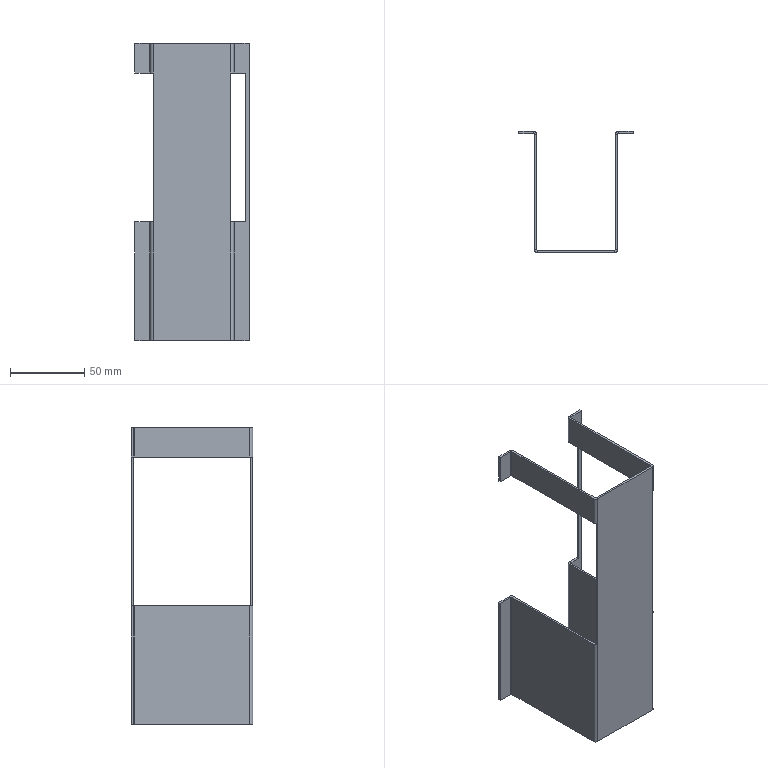Part | STEP file | B1-029 | 1 solid | 70 faces | box 77 x 81.5 x 200 mm | volume 43403 mm3 | plane 54 | cylinder 16 | commonest cylinder face diameters 1 x8 4 x8